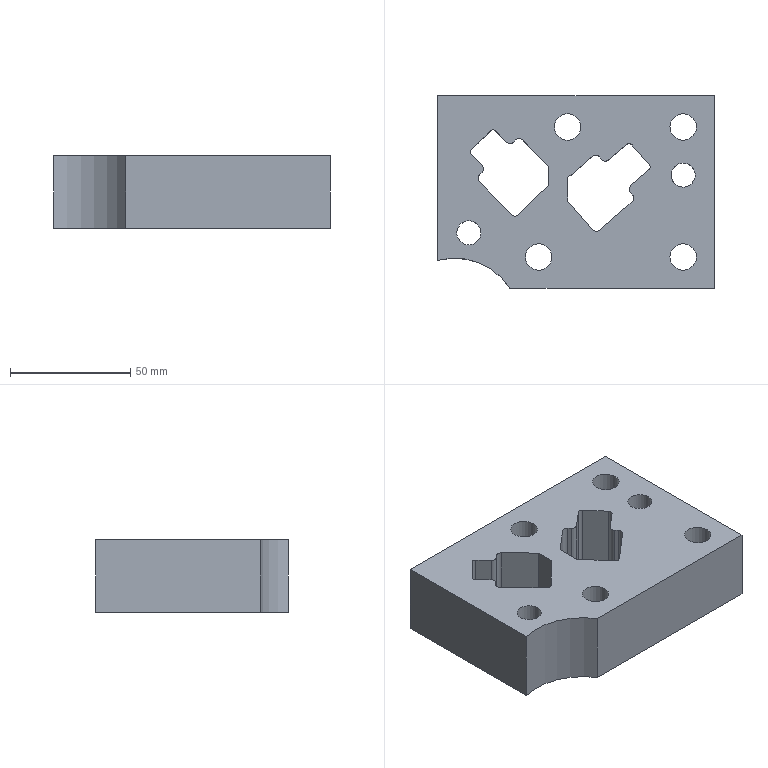Part | STEP file | 215_id698_x_t | 1 solid | 57 faces | box 115 x 80 x 30 mm | volume 200547 mm3 | plane 28 | cylinder 27 | other 1 | spline 1 | commonest cylinder face diameters 4 x10 11 x6 3 x4 17 x4 10 x2 55 x1